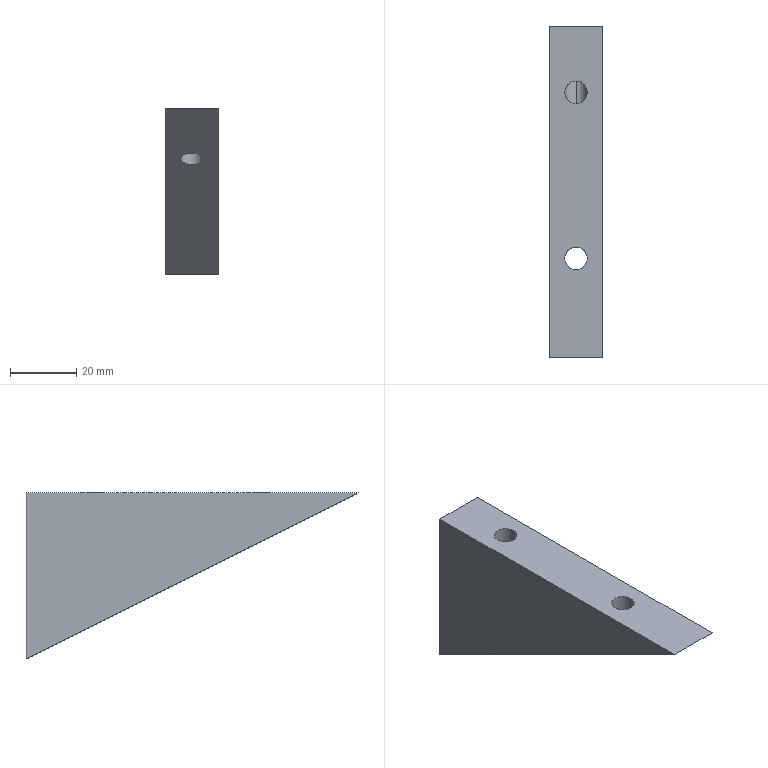Part | SolidWorks | features HoleWzd 2, Extrusion 1 | 1 solid | 16 faces | box 16 x 100 x 50 mm | volume 37384 mm3 | cylinder 6 | cone 5 | plane 5 | commonest cylinder face diameters 6.8 x6
STEP:
#1=CARTESIAN_POINT('',(11.326,-20.,-29.294));
#2=VERTEX_POINT('',#1);
#3=CARTESIAN_POINT('',(11.316,-19.25,-29.25));
#4=VERTEX_POINT('',#3);
#5=CARTESIAN_POINT('',(11.326,-20.,-29.294));
#6=CARTESIAN_POINT('',(11.326,-19.75,-29.294));
#7=CARTESIAN_POINT('',(11.323,-19.498,-29.279));
#8=CARTESIAN_POINT('',(11.316,-19.25,-29.25));
#9=B_SPLINE_CURVE_WITH_KNOTS('',3,(#5,#6,#7,#8),.UNSPECIFIED.,.F.,.F.,(4,4),(0.001846,0.002591),.UNSPECIFIED.);
#10=EDGE_CURVE('',#2,#4,#9,.T.);
#11=ORIENTED_EDGE('',*,*,#10,.F.);
#12=CARTESIAN_POINT('',(11.4,-20.,-29.25));
#13=VERTEX_POINT('',#12);
#14=CARTESIAN_POINT('',(11.4,-20.,-29.25));
#15=DIRECTION('',(0.8572,0.,0.515));
#16=VECTOR('',#15,1000.);
#17=LINE('',#14,#16);
#18=EDGE_CURVE('',#2,#13,#17,.T.);
#19=ORIENTED_EDGE('',*,*,#18,.T.);
#20=CARTESIAN_POINT('',(8.,-20.,-29.25));
#21=DIRECTION('',(0.,0.,1.));
#22=DIRECTION('',(1.,0.,0.));
#23=AXIS2_PLACEMENT_3D('',#20,#21,#22);
#24=CIRCLE('',#23,3.4);
#25=EDGE_CURVE('',#13,#4,#24,.T.);
#26=ORIENTED_EDGE('',*,*,#25,.T.);
#27=EDGE_LOOP('',(#11,#19,#26));
#28=FACE_OUTER_BOUND('',#27,.T.);
#29=CARTESIAN_POINT('',(8.,-20.,-29.25));
#30=DIRECTION('',(0.,0.,1.));
#31=DIRECTION('',(1.,0.,0.));
#32=AXIS2_PLACEMENT_3D('',#29,#30,#31);
#33=CONICAL_SURFACE('',#32,3.4,1.03);
#34=ADVANCED_FACE('',(#28),#33,.F.);
#35=CARTESIAN_POINT('',(4.6,-20.,-29.25));
#36=VERTEX_POINT('',#35);
#37=CARTESIAN_POINT('',(4.684,-20.75,-29.25));
#38=VERTEX_POINT('',#37);
#39=CARTESIAN_POINT('',(8.,-20.,-29.25));
#40=DIRECTION('',(0.,0.,1.));
#41=DIRECTION('',(1.,0.,0.));
#42=AXIS2_PLACEMENT_3D('',#39,#40,#41);
#43=CIRCLE('',#42,3.4);
#44=EDGE_CURVE('',#36,#38,#43,.T.);
#45=ORIENTED_EDGE('',*,*,#44,.F.);
#46=CARTESIAN_POINT('',(4.6,-20.,0.));
#47=VERTEX_POINT('',#46);
#48=CARTESIAN_POINT('',(4.6,-20.,0.));
#49=DIRECTION('',(0.,0.,1.));
#50=VECTOR('',#49,1000.);
#51=LINE('',#48,#50);
#52=EDGE_CURVE('',#36,#47,#51,.T.);
#53=ORIENTED_EDGE('',*,*,#52,.T.);
#54=CARTESIAN_POINT('',(11.4,-20.,0.));
#55=VERTEX_POINT('',#54);
#56=CARTESIAN_POINT('',(8.,-20.,0.));
#57=DIRECTION('',(0.,0.,1.));
#58=DIRECTION('',(1.,0.,0.));
#59=AXIS2_PLACEMENT_3D('',#56,#57,#58);
#60=CIRCLE('',#59,3.4);
#61=EDGE_CURVE('',#47,#55,#60,.T.);
#62=ORIENTED_EDGE('',*,*,#61,.T.);
#63=CARTESIAN_POINT('',(11.4,-20.,0.));
#64=DIRECTION('',(0.,0.,1.));
#65=VECTOR('',#64,1000.);
#66=LINE('',#63,#65);
#67=EDGE_CURVE('',#13,#55,#66,.T.);
#68=ORIENTED_EDGE('',*,*,#67,.F.);
#69=CARTESIAN_POINT('',(11.316,-20.75,-29.25));
#70=VERTEX_POINT('',#69);
#71=CARTESIAN_POINT('',(8.,-20.,-29.25));
#72=DIRECTION('',(0.,0.,1.));
#73=DIRECTION('',(1.,0.,0.));
#74=AXIS2_PLACEMENT_3D('',#71,#72,#73);
#75=CIRCLE('',#74,3.4);
#76=EDGE_CURVE('',#70,#13,#75,.T.);
#77=ORIENTED_EDGE('',*,*,#76,.F.);
#78=CARTESIAN_POINT('',(8.,-23.4,-26.6));
#79=VERTEX_POINT('',#78);
#80=CARTESIAN_POINT('',(8.,-23.4,-26.6));
#81=CARTESIAN_POINT('',(9.657,-23.4,-26.6));
#82=CARTESIAN_POINT('',(10.951,-22.366,-27.634));
#83=CARTESIAN_POINT('',(11.316,-20.75,-29.25));
#84=(BOUNDED_CURVE()B_SPLINE_CURVE(3,(#80,#81,#82,#83),.UNSPECIFIED.,.F.,.F.)B_SPLINE_CURVE_WITH_KNOTS((4,4),(3.142,4.49),.UNSPECIFIED.)CURVE()GEOMETRIC_REPRESENTATION_ITEM()RATIONAL_B_SPLINE_CURVE((1.,0.8541,0.8541,1.))REPRESENTATION_ITEM(''));
#85=EDGE_CURVE('',#79,#70,#84,.T.);
#86=ORIENTED_EDGE('',*,*,#85,.F.);
#87=CARTESIAN_POINT('',(4.684,-20.75,-29.25));
#88=CARTESIAN_POINT('',(5.049,-22.366,-27.634));
#89=CARTESIAN_POINT('',(6.343,-23.4,-26.6));
#90=CARTESIAN_POINT('',(8.,-23.4,-26.6));
#91=(BOUNDED_CURVE()B_SPLINE_CURVE(3,(#87,#88,#89,#90),.UNSPECIFIED.,.F.,.F.)B_SPLINE_CURVE_WITH_KNOTS((4,4),(1.793,3.142),.UNSPECIFIED.)CURVE()GEOMETRIC_REPRESENTATION_ITEM()RATIONAL_B_SPLINE_CURVE((1.,0.8541,0.8541,1.))REPRESENTATION_ITEM(''));
#92=EDGE_CURVE('',#38,#79,#91,.T.);
#93=ORIENTED_EDGE('',*,*,#92,.F.);
#94=EDGE_LOOP('',(#45,#53,#62,#68,#77,#86,#93));
#95=FACE_OUTER_BOUND('',#94,.T.);
#96=CARTESIAN_POINT('',(8.,-20.,0.));
#97=DIRECTION('',(0.,0.,1.));
#98=DIRECTION('',(1.,0.,0.));
#99=AXIS2_PLACEMENT_3D('',#96,#97,#98);
#100=CYLINDRICAL_SURFACE('',#99,3.4);
#101=ADVANCED_FACE('',(#95),#100,.F.);
#102=CARTESIAN_POINT('',(4.6,-70.,-15.));
#103=VERTEX_POINT('',#102);
#104=CARTESIAN_POINT('',(11.4,-70.,-15.));
#105=VERTEX_POINT('',#104);
#106=CARTESIAN_POINT('',(4.6,-70.,-15.));
#107=CARTESIAN_POINT('',(4.6,-76.8,-11.6));
#108=CARTESIAN_POINT('',(11.4,-76.8,-11.6));
#109=CARTESIAN_POINT('',(11.4,-70.,-15.));
#110=(BOUNDED_CURVE()B_SPLINE_CURVE(3,(#106,#107,#108,#109),.UNSPECIFIED.,.F.,.F.)B_SPLINE_CURVE_WITH_KNOTS((4,4),(4.712,7.854),.UNSPECIFIED.)CURVE()GEOMETRIC_REPRESENTATION_ITEM()RATIONAL_B_SPLINE_CURVE((1.,0.3333,0.3333,1.))REPRESENTATION_ITEM(''));
#111=EDGE_CURVE('',#103,#105,#110,.T.);
#112=ORIENTED_EDGE('',*,*,#111,.F.);
#113=CARTESIAN_POINT('',(4.6,-70.,0.));
#114=VERTEX_POINT('',#113);
#115=CARTESIAN_POINT('',(4.6,-70.,0.));
#116=DIRECTION('',(0.,0.,1.));
#117=VECTOR('',#116,1000.);
#118=LINE('',#115,#117);
#119=EDGE_CURVE('',#103,#114,#118,.T.);
#120=ORIENTED_EDGE('',*,*,#119,.T.);
#121=CARTESIAN_POINT('',(11.4,-70.,0.));
#122=VERTEX_POINT('',#121);
#123=CARTESIAN_POINT('',(8.,-70.,0.));
#124=DIRECTION('',(0.,0.,1.));
#125=DIRECTION('',(1.,0.,0.));
#126=AXIS2_PLACEMENT_3D('',#123,#124,#125);
#127=CIRCLE('',#126,3.4);
#128=EDGE_CURVE('',#114,#122,#127,.T.);
#129=ORIENTED_EDGE('',*,*,#128,.T.);
#130=CARTESIAN_POINT('',(11.4,-70.,0.));
#131=DIRECTION('',(0.,0.,1.));
#132=VECTOR('',#131,1000.);
#133=LINE('',#130,#132);
#134=EDGE_CURVE('',#105,#122,#133,.T.);
#135=ORIENTED_EDGE('',*,*,#134,.F.);
#136=EDGE_LOOP('',(#112,#120,#129,#135));
#137=FACE_OUTER_BOUND('',#136,.T.);
#138=CARTESIAN_POINT('',(8.,-70.,0.));
#139=DIRECTION('',(0.,0.,1.));
#140=DIRECTION('',(1.,0.,0.));
#141=AXIS2_PLACEMENT_3D('',#138,#139,#140);
#142=CYLINDRICAL_SURFACE('',#141,3.4);
#143=ADVANCED_FACE('',(#137),#142,.F.);
#144=CARTESIAN_POINT('',(8.,-29.25,-33.4));
#145=VERTEX_POINT('',#144);
#146=CARTESIAN_POINT('',(8.,-29.25,-26.6));
#147=VERTEX_POINT('',#146);
#148=CARTESIAN_POINT('',(8.,-29.25,-30.));
#149=DIRECTION('',(0.,1.,0.));
#150=DIRECTION('',(0.,0.,1.));
#151=AXIS2_PLACEMENT_3D('',#148,#149,#150);
#152=CIRCLE('',#151,3.4);
#153=EDGE_CURVE('',#145,#147,#152,.T.);
#154=ORIENTED_EDGE('',*,*,#153,.F.);
#155=CARTESIAN_POINT('',(8.,0.,-33.4));
#156=VERTEX_POINT('',#155);
#157=CARTESIAN_POINT('',(8.,0.,-33.4));
#158=DIRECTION('',(0.,1.,0.));
#159=VECTOR('',#158,1000.);
#160=LINE('',#157,#159);
#161=EDGE_CURVE('',#145,#156,#160,.T.);
#162=ORIENTED_EDGE('',*,*,#161,.T.);
#163=CARTESIAN_POINT('',(8.,0.,-26.6));
#164=VERTEX_POINT('',#163);
#165=CARTESIAN_POINT('',(8.,0.,-30.));
#166=DIRECTION('',(0.,1.,0.));
#167=DIRECTION('',(0.,0.,1.));
#168=AXIS2_PLACEMENT_3D('',#165,#166,#167);
#169=CIRCLE('',#168,3.4);
#170=EDGE_CURVE('',#156,#164,#169,.T.);
#171=ORIENTED_EDGE('',*,*,#170,.T.);
#172=CARTESIAN_POINT('',(8.,-16.6,-26.6));
#173=VERTEX_POINT('',#172);
#174=CARTESIAN_POINT('',(8.,0.,-26.6));
#175=DIRECTION('',(0.,1.,0.));
#176=VECTOR('',#175,1000.);
#177=LINE('',#174,#176);
#178=EDGE_CURVE('',#173,#164,#177,.T.);
#179=ORIENTED_EDGE('',*,*,#178,.F.);
#180=CARTESIAN_POINT('',(4.684,-19.25,-29.25));
#181=VERTEX_POINT('',#180);
#182=CARTESIAN_POINT('',(8.,-16.6,-26.6));
#183=CARTESIAN_POINT('',(6.343,-16.6,-26.6));
#184=CARTESIAN_POINT('',(5.049,-17.634,-27.634));
#185=CARTESIAN_POINT('',(4.684,-19.25,-29.25));
#186=(BOUNDED_CURVE()B_SPLINE_CURVE(3,(#182,#183,#184,#185),.UNSPECIFIED.,.F.,.F.)B_SPLINE_CURVE_WITH_KNOTS((4,4),(0.,1.348),.UNSPECIFIED.)CURVE()GEOMETRIC_REPRESENTATION_ITEM()RATIONAL_B_SPLINE_CURVE((1.,0.8541,0.8541,1.))REPRESENTATION_ITEM(''));
#187=EDGE_CURVE('',#173,#181,#186,.T.);
#188=ORIENTED_EDGE('',*,*,#187,.T.);
#189=CARTESIAN_POINT('',(4.684,-19.25,-29.25));
#190=CARTESIAN_POINT('',(4.677,-19.497,-29.279));
#191=CARTESIAN_POINT('',(4.674,-19.747,-29.294));
#192=CARTESIAN_POINT('',(4.674,-20.249,-29.295));
#193=CARTESIAN_POINT('',(4.677,-20.501,-29.279));
#194=CARTESIAN_POINT('',(4.684,-20.75,-29.25));
#195=B_SPLINE_CURVE_WITH_KNOTS('',3,(#189,#190,#191,#192,#193,#194),.UNSPECIFIED.,.F.,.F.,(4,2,4),(0.001096,0.001843,0.002591),.UNSPECIFIED.);
#196=EDGE_CURVE('',#181,#38,#195,.T.);
#197=ORIENTED_EDGE('',*,*,#196,.T.);
#198=ORIENTED_EDGE('',*,*,#92,.T.);
#199=CARTESIAN_POINT('',(8.,0.,-26.6));
#200=DIRECTION('',(0.,1.,0.));
#201=VECTOR('',#200,1000.);
#202=LINE('',#199,#201);
#203=EDGE_CURVE('',#147,#79,#202,.T.);
#204=ORIENTED_EDGE('',*,*,#203,.F.);
#205=EDGE_LOOP('',(#154,#162,#171,#179,#188,#197,#198,#204));
#206=FACE_OUTER_BOUND('',#205,.T.);
#207=CARTESIAN_POINT('',(8.,0.,-30.));
#208=DIRECTION('',(0.,1.,0.));
#209=DIRECTION('',(0.,0.,1.));
#210=AXIS2_PLACEMENT_3D('',#207,#208,#209);
#211=CYLINDRICAL_SURFACE('',#210,3.4);
#212=ADVANCED_FACE('',(#206),#211,.F.);
#213=CARTESIAN_POINT('',(8.,-31.293,-30.));
#214=VERTEX_POINT('',#213);
#215=CARTESIAN_POINT('',(8.,-29.25,-26.6));
#216=DIRECTION('',(0.,0.515,0.8572));
#217=VECTOR('',#216,1000.);
#218=LINE('',#215,#217);
#219=EDGE_CURVE('',#214,#147,#218,.T.);
#220=ORIENTED_EDGE('',*,*,#219,.F.);
#221=CARTESIAN_POINT('',(8.,-29.25,-33.4));
#222=DIRECTION('',(0.,0.515,-0.8572));
#223=VECTOR('',#222,1000.);
#224=LINE('',#221,#223);
#225=EDGE_CURVE('',#214,#145,#224,.T.);
#226=ORIENTED_EDGE('',*,*,#225,.T.);
#227=ORIENTED_EDGE('',*,*,#153,.T.);
#228=EDGE_LOOP('',(#220,#226,#227));
#229=FACE_OUTER_BOUND('',#228,.T.);
#230=CARTESIAN_POINT('',(8.,-29.25,-30.));
#231=DIRECTION('',(0.,1.,0.));
#232=DIRECTION('',(0.,0.,1.));
#233=AXIS2_PLACEMENT_3D('',#230,#231,#232);
#234=CONICAL_SURFACE('',#233,3.4,1.03);
#235=ADVANCED_FACE('',(#229),#234,.F.);
#236=CARTESIAN_POINT('',(8.,-20.,0.));
#237=DIRECTION('',(0.,0.,1.));
#238=DIRECTION('',(1.,0.,0.));
#239=AXIS2_PLACEMENT_3D('',#236,#237,#238);
#240=CIRCLE('',#239,3.4);
#241=EDGE_CURVE('',#55,#47,#240,.T.);
#242=ORIENTED_EDGE('',*,*,#241,.F.);
#243=ORIENTED_EDGE('',*,*,#61,.F.);
#244=EDGE_LOOP('',(#242,#243));
#245=FACE_BOUND('',#244,.T.);
#246=CARTESIAN_POINT('',(8.,-70.,0.));
#247=DIRECTION('',(0.,0.,1.));
#248=DIRECTION('',(1.,0.,0.));
#249=AXIS2_PLACEMENT_3D('',#246,#247,#248);
#250=CIRCLE('',#249,3.4);
#251=EDGE_CURVE('',#122,#114,#250,.T.);
#252=ORIENTED_EDGE('',*,*,#251,.F.);
#253=ORIENTED_EDGE('',*,*,#128,.F.);
#254=EDGE_LOOP('',(#252,#253));
#255=FACE_BOUND('',#254,.T.);
#256=CARTESIAN_POINT('',(0.,0.,0.));
#257=VERTEX_POINT('',#256);
#258=CARTESIAN_POINT('',(0.,-100.,0.));
#259=VERTEX_POINT('',#258);
#260=CARTESIAN_POINT('',(0.,-100.,0.));
#261=DIRECTION('',(0.,-1.,0.));
#262=VECTOR('',#261,1000.);
#263=LINE('',#260,#262);
#264=EDGE_CURVE('',#257,#259,#263,.T.);
#265=ORIENTED_EDGE('',*,*,#264,.T.);
#266=CARTESIAN_POINT('',(16.,-100.,0.));
#267=VERTEX_POINT('',#266);
#268=CARTESIAN_POINT('',(16.,-100.,0.));
#269=DIRECTION('',(-1.,0.,0.));
#270=VECTOR('',#269,1000.);
#271=LINE('',#268,#270);
#272=EDGE_CURVE('',#267,#259,#271,.T.);
#273=ORIENTED_EDGE('',*,*,#272,.F.);
#274=CARTESIAN_POINT('',(16.,0.,0.));
#275=VERTEX_POINT('',#274);
#276=CARTESIAN_POINT('',(16.,-100.,0.));
#277=DIRECTION('',(0.,-1.,0.));
#278=VECTOR('',#277,1000.);
#279=LINE('',#276,#278);
#280=EDGE_CURVE('',#275,#267,#279,.T.);
#281=ORIENTED_EDGE('',*,*,#280,.F.);
#282=CARTESIAN_POINT('',(16.,0.,0.));
#283=DIRECTION('',(-1.,0.,0.));
#284=VECTOR('',#283,1000.);
#285=LINE('',#282,#284);
#286=EDGE_CURVE('',#275,#257,#285,.T.);
#287=ORIENTED_EDGE('',*,*,#286,.T.);
#288=EDGE_LOOP('',(#265,#273,#281,#287));
#289=FACE_OUTER_BOUND('',#288,.T.);
#290=CARTESIAN_POINT('',(16.,-100.,0.));
#291=DIRECTION('',(0.,0.,-1.));
#292=DIRECTION('',(-1.,0.,0.));
#293=AXIS2_PLACEMENT_3D('',#290,#291,#292);
#294=PLANE('',#293);
#295=ADVANCED_FACE('',(#245,#255,#289),#294,.F.);
#296=CARTESIAN_POINT('',(11.4,-70.,-15.));
#297=CARTESIAN_POINT('',(11.4,-63.2,-18.4));
#298=CARTESIAN_POINT('',(4.6,-63.2,-18.4));
#299=CARTESIAN_POINT('',(4.6,-70.,-15.));
#300=(BOUNDED_CURVE()B_SPLINE_CURVE(3,(#296,#297,#298,#299),.UNSPECIFIED.,.F.,.F.)B_SPLINE_CURVE_WITH_KNOTS((4,4),(1.571,4.712),.UNSPECIFIED.)CURVE()GEOMETRIC_REPRESENTATION_ITEM()RATIONAL_B_SPLINE_CURVE((1.,0.3333,0.3333,1.))REPRESENTATION_ITEM(''));
#301=EDGE_CURVE('',#105,#103,#300,.T.);
#302=ORIENTED_EDGE('',*,*,#301,.T.);
#303=ORIENTED_EDGE('',*,*,#111,.T.);
#304=EDGE_LOOP('',(#302,#303));
#305=FACE_BOUND('',#304,.T.);
#306=CARTESIAN_POINT('',(0.,0.,-50.));
#307=VERTEX_POINT('',#306);
#308=CARTESIAN_POINT('',(0.,0.,-50.));
#309=DIRECTION('',(0.,0.8944,-0.4472));
#310=VECTOR('',#309,1000.);
#311=LINE('',#308,#310);
#312=EDGE_CURVE('',#259,#307,#311,.T.);
#313=ORIENTED_EDGE('',*,*,#312,.T.);
#314=CARTESIAN_POINT('',(16.,0.,-50.));
#315=VERTEX_POINT('',#314);
#316=CARTESIAN_POINT('',(16.,0.,-50.));
#317=DIRECTION('',(-1.,0.,0.));
#318=VECTOR('',#317,1000.);
#319=LINE('',#316,#318);
#320=EDGE_CURVE('',#315,#307,#319,.T.);
#321=ORIENTED_EDGE('',*,*,#320,.F.);
#322=CARTESIAN_POINT('',(16.,0.,-50.));
#323=DIRECTION('',(0.,0.8944,-0.4472));
#324=VECTOR('',#323,1000.);
#325=LINE('',#322,#324);
#326=EDGE_CURVE('',#267,#315,#325,.T.);
#327=ORIENTED_EDGE('',*,*,#326,.F.);
#328=ORIENTED_EDGE('',*,*,#272,.T.);
#329=EDGE_LOOP('',(#313,#321,#327,#328));
#330=FACE_OUTER_BOUND('',#329,.T.);
#331=CARTESIAN_POINT('',(16.,0.,-50.));
#332=DIRECTION('',(0.,0.4472,0.8944));
#333=DIRECTION('',(0.,-0.8944,0.4472));
#334=AXIS2_PLACEMENT_3D('',#331,#332,#333);
#335=PLANE('',#334);
#336=ADVANCED_FACE('',(#305,#330),#335,.F.);
#337=CARTESIAN_POINT('',(8.,0.,-30.));
#338=DIRECTION('',(0.,1.,0.));
#339=DIRECTION('',(0.,0.,1.));
#340=AXIS2_PLACEMENT_3D('',#337,#338,#339);
#341=CIRCLE('',#340,3.4);
#342=EDGE_CURVE('',#164,#156,#341,.T.);
#343=ORIENTED_EDGE('',*,*,#342,.F.);
#344=ORIENTED_EDGE('',*,*,#170,.F.);
#345=EDGE_LOOP('',(#343,#344));
#346=FACE_BOUND('',#345,.T.);
#347=CARTESIAN_POINT('',(0.,0.,0.));
#348=DIRECTION('',(0.,0.,1.));
#349=VECTOR('',#348,1000.);
#350=LINE('',#347,#349);
#351=EDGE_CURVE('',#307,#257,#350,.T.);
#352=ORIENTED_EDGE('',*,*,#351,.T.);
#353=ORIENTED_EDGE('',*,*,#286,.F.);
#354=CARTESIAN_POINT('',(16.,0.,0.));
#355=DIRECTION('',(0.,0.,1.));
#356=VECTOR('',#355,1000.);
#357=LINE('',#354,#356);
#358=EDGE_CURVE('',#315,#275,#357,.T.);
#359=ORIENTED_EDGE('',*,*,#358,.F.);
#360=ORIENTED_EDGE('',*,*,#320,.T.);
#361=EDGE_LOOP('',(#352,#353,#359,#360));
#362=FACE_OUTER_BOUND('',#361,.T.);
#363=CARTESIAN_POINT('',(16.,0.,0.));
#364=DIRECTION('',(0.,-1.,0.));
#365=DIRECTION('',(0.,0.,-1.));
#366=AXIS2_PLACEMENT_3D('',#363,#364,#365);
#367=PLANE('',#366);
#368=ADVANCED_FACE('',(#346,#362),#367,.F.);
#369=ORIENTED_EDGE('',*,*,#280,.T.);
#370=ORIENTED_EDGE('',*,*,#326,.T.);
#371=ORIENTED_EDGE('',*,*,#358,.T.);
#372=EDGE_LOOP('',(#369,#370,#371));
#373=FACE_OUTER_BOUND('',#372,.T.);
#374=CARTESIAN_POINT('',(16.,0.,0.));
#375=DIRECTION('',(-1.,0.,0.));
#376=DIRECTION('',(0.,0.,1.));
#377=AXIS2_PLACEMENT_3D('',#374,#375,#376);
#378=PLANE('',#377);
#379=ADVANCED_FACE('',(#373),#378,.F.);
#380=ORIENTED_EDGE('',*,*,#264,.F.);
#381=ORIENTED_EDGE('',*,*,#351,.F.);
#382=ORIENTED_EDGE('',*,*,#312,.F.);
#383=EDGE_LOOP('',(#380,#381,#382));
#384=FACE_OUTER_BOUND('',#383,.T.);
#385=CARTESIAN_POINT('',(0.,0.,0.));
#386=DIRECTION('',(-1.,0.,0.));
#387=DIRECTION('',(0.,0.,1.));
#388=AXIS2_PLACEMENT_3D('',#385,#386,#387);
#389=PLANE('',#388);
#390=ADVANCED_FACE('',(#384),#389,.T.);
#391=ORIENTED_EDGE('',*,*,#225,.F.);
#392=ORIENTED_EDGE('',*,*,#219,.T.);
#393=CARTESIAN_POINT('',(8.,-29.25,-30.));
#394=DIRECTION('',(0.,1.,0.));
#395=DIRECTION('',(0.,0.,1.));
#396=AXIS2_PLACEMENT_3D('',#393,#394,#395);
#397=CIRCLE('',#396,3.4);
#398=EDGE_CURVE('',#147,#145,#397,.T.);
#399=ORIENTED_EDGE('',*,*,#398,.T.);
#400=EDGE_LOOP('',(#391,#392,#399));
#401=FACE_OUTER_BOUND('',#400,.T.);
#402=CARTESIAN_POINT('',(8.,-29.25,-30.));
#403=DIRECTION('',(0.,1.,0.));
#404=DIRECTION('',(0.,0.,1.));
#405=AXIS2_PLACEMENT_3D('',#402,#403,#404);
#406=CONICAL_SURFACE('',#405,3.4,1.03);
#407=ADVANCED_FACE('',(#401),#406,.F.);
#408=ORIENTED_EDGE('',*,*,#161,.F.);
#409=ORIENTED_EDGE('',*,*,#398,.F.);
#410=ORIENTED_EDGE('',*,*,#203,.T.);
#411=ORIENTED_EDGE('',*,*,#85,.T.);
#412=CARTESIAN_POINT('',(11.316,-20.75,-29.25));
#413=CARTESIAN_POINT('',(11.323,-20.502,-29.279));
#414=CARTESIAN_POINT('',(11.326,-20.252,-29.294));
#415=CARTESIAN_POINT('',(11.326,-20.,-29.294));
#416=B_SPLINE_CURVE_WITH_KNOTS('',3,(#412,#413,#414,#415),.UNSPECIFIED.,.F.,.F.,(4,4),(0.001096,0.001846),.UNSPECIFIED.);
#417=EDGE_CURVE('',#70,#2,#416,.T.);
#418=ORIENTED_EDGE('',*,*,#417,.T.);
#419=ORIENTED_EDGE('',*,*,#10,.T.);
#420=CARTESIAN_POINT('',(11.316,-19.25,-29.25));
#421=CARTESIAN_POINT('',(10.951,-17.634,-27.634));
#422=CARTESIAN_POINT('',(9.657,-16.6,-26.6));
#423=CARTESIAN_POINT('',(8.,-16.6,-26.6));
#424=(BOUNDED_CURVE()B_SPLINE_CURVE(3,(#420,#421,#422,#423),.UNSPECIFIED.,.F.,.F.)B_SPLINE_CURVE_WITH_KNOTS((4,4),(4.935,6.283),.UNSPECIFIED.)CURVE()GEOMETRIC_REPRESENTATION_ITEM()RATIONAL_B_SPLINE_CURVE((1.,0.8541,0.8541,1.))REPRESENTATION_ITEM(''));
#425=EDGE_CURVE('',#4,#173,#424,.T.);
#426=ORIENTED_EDGE('',*,*,#425,.T.);
#427=ORIENTED_EDGE('',*,*,#178,.T.);
#428=ORIENTED_EDGE('',*,*,#342,.T.);
#429=EDGE_LOOP('',(#408,#409,#410,#411,#418,#419,#426,#427,#428));
#430=FACE_OUTER_BOUND('',#429,.T.);
#431=CARTESIAN_POINT('',(8.,0.,-30.));
#432=DIRECTION('',(0.,1.,0.));
#433=DIRECTION('',(0.,0.,1.));
#434=AXIS2_PLACEMENT_3D('',#431,#432,#433);
#435=CYLINDRICAL_SURFACE('',#434,3.4);
#436=ADVANCED_FACE('',(#430),#435,.F.);
#437=ORIENTED_EDGE('',*,*,#119,.F.);
#438=ORIENTED_EDGE('',*,*,#301,.F.);
#439=ORIENTED_EDGE('',*,*,#134,.T.);
#440=ORIENTED_EDGE('',*,*,#251,.T.);
#441=EDGE_LOOP('',(#437,#438,#439,#440));
#442=FACE_OUTER_BOUND('',#441,.T.);
#443=CARTESIAN_POINT('',(8.,-70.,0.));
#444=DIRECTION('',(0.,0.,1.));
#445=DIRECTION('',(1.,0.,0.));
#446=AXIS2_PLACEMENT_3D('',#443,#444,#445);
#447=CYLINDRICAL_SURFACE('',#446,3.4);
#448=ADVANCED_FACE('',(#442),#447,.F.);
#449=ORIENTED_EDGE('',*,*,#52,.F.);
#450=CARTESIAN_POINT('',(8.,-20.,-29.25));
#451=DIRECTION('',(0.,0.,1.));
#452=DIRECTION('',(1.,0.,0.));
#453=AXIS2_PLACEMENT_3D('',#450,#451,#452);
#454=CIRCLE('',#453,3.4);
#455=EDGE_CURVE('',#181,#36,#454,.T.);
#456=ORIENTED_EDGE('',*,*,#455,.F.);
#457=ORIENTED_EDGE('',*,*,#187,.F.);
#458=ORIENTED_EDGE('',*,*,#425,.F.);
#459=ORIENTED_EDGE('',*,*,#25,.F.);
#460=ORIENTED_EDGE('',*,*,#67,.T.);
#461=ORIENTED_EDGE('',*,*,#241,.T.);
#462=EDGE_LOOP('',(#449,#456,#457,#458,#459,#460,#461));
#463=FACE_OUTER_BOUND('',#462,.T.);
#464=CARTESIAN_POINT('',(8.,-20.,0.));
#465=DIRECTION('',(0.,0.,1.));
#466=DIRECTION('',(1.,0.,0.));
#467=AXIS2_PLACEMENT_3D('',#464,#465,#466);
#468=CYLINDRICAL_SURFACE('',#467,3.4);
#469=ADVANCED_FACE('',(#463),#468,.F.);
#470=ORIENTED_EDGE('',*,*,#18,.F.);
#471=ORIENTED_EDGE('',*,*,#417,.F.);
#472=ORIENTED_EDGE('',*,*,#76,.T.);
#473=EDGE_LOOP('',(#470,#471,#472));
#474=FACE_OUTER_BOUND('',#473,.T.);
#475=CARTESIAN_POINT('',(8.,-20.,-29.25));
#476=DIRECTION('',(0.,0.,1.));
#477=DIRECTION('',(1.,0.,0.));
#478=AXIS2_PLACEMENT_3D('',#475,#476,#477);
#479=CONICAL_SURFACE('',#478,3.4,1.03);
#480=ADVANCED_FACE('',(#474),#479,.F.);
#481=ORIENTED_EDGE('',*,*,#455,.T.);
#482=ORIENTED_EDGE('',*,*,#44,.T.);
#483=ORIENTED_EDGE('',*,*,#196,.F.);
#484=EDGE_LOOP('',(#481,#482,#483));
#485=FACE_OUTER_BOUND('',#484,.T.);
#486=CARTESIAN_POINT('',(8.,-20.,-29.25));
#487=DIRECTION('',(0.,0.,1.));
#488=DIRECTION('',(1.,0.,0.));
#489=AXIS2_PLACEMENT_3D('',#486,#487,#488);
#490=CONICAL_SURFACE('',#489,3.4,1.03);
#491=ADVANCED_FACE('',(#485),#490,.F.);
#492=CLOSED_SHELL('',(#34,#101,#143,#212,#235,#295,#336,#368,#379,#390,#407,#436,#448,#469,#480,#491));
#493=MANIFOLD_SOLID_BREP('',#492);
#494=CARTESIAN_POINT('',(0.,0.,0.));
#495=DIRECTION('',(0.,0.,1.));
#496=DIRECTION('',(1.,0.,0.));
#497=AXIS2_PLACEMENT_3D('',#494,#495,#496);
#498=(LENGTH_UNIT()NAMED_UNIT(*)SI_UNIT(.MILLI.,.METRE.));
#499=UNCERTAINTY_MEASURE_WITH_UNIT(LENGTH_MEASURE(0.00001),#498,'','');
#500=(NAMED_UNIT(*)PLANE_ANGLE_UNIT()SI_UNIT($,.RADIAN.));
#501=(NAMED_UNIT(*)SI_UNIT($,.STERADIAN.)SOLID_ANGLE_UNIT());
#502=(GEOMETRIC_REPRESENTATION_CONTEXT(3)GLOBAL_UNCERTAINTY_ASSIGNED_CONTEXT((#499))GLOBAL_UNIT_ASSIGNED_CONTEXT((#498,#500,#501))REPRESENTATION_CONTEXT('',''));
#503=ADVANCED_BREP_SHAPE_REPRESENTATION('',(#493,#497),#502);